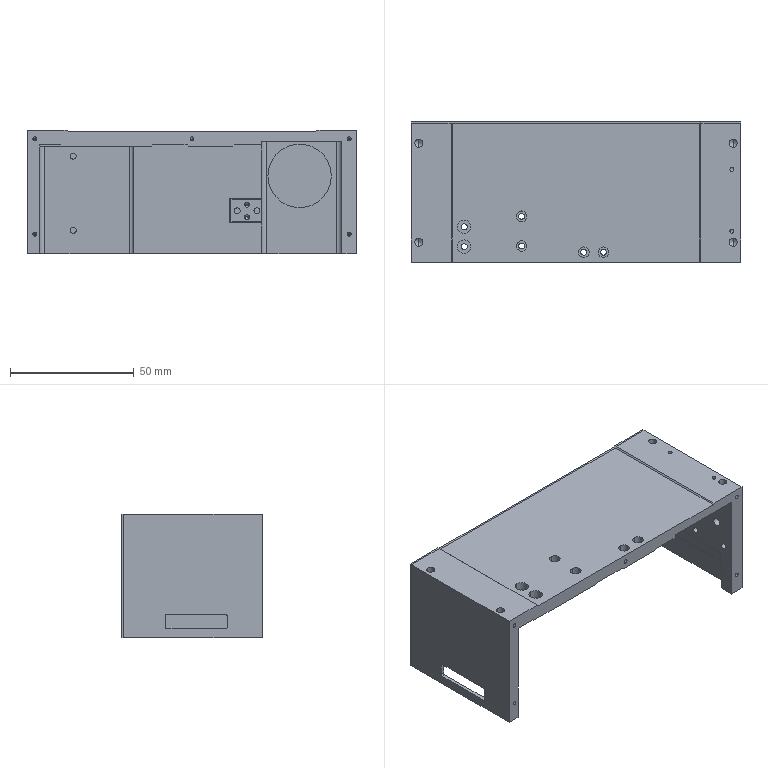NC program | NX | posted with a generic post | part box 133 x 56.74 x 50 mm
Lines 6286 to 7308 of 22463:
(CAVITY_MILL_COPY , TOOL : D6)
N12546 T06 M6
N12548 G54
N12550 G17 G0 G90 X58.566 Y-14.571 B0. C0. S9509 M3
N12552 G43 Z30. H6
N12554 Z1.
N12556 G94 G1 Z-0.5 F1000.
N12558 X59.504 Y-15.367
N12560 G3 X60.488 Y-15.546 R1.
N12562 G2 X61.5 Y-15.37 R3. F1500.
N12564 G1 X62.
N12566 Y-13.594
N12568 G3 X61.5 Y-12.728 R1.
N12570 G1 X60.2 Y-11.977
N12572 Z1.
N12574 G0 Z30.
N12576 X58.566 Y-14.571
N12578 Z0.5
N12580 G1 Z-1. F1000.
N12582 X59.504 Y-15.367
N12584 G3 X60.488 Y-15.546 R1.
N12586 G2 X61.5 Y-15.37 R3. F1500.
N12588 G1 X62.
N12590 Y-13.594
N12592 G3 X61.5 Y-12.728 R1.
N12594 G1 X60.2 Y-11.977
N12596 Z0.5
N12598 G0 Z30.
N12600 X58.566 Y-14.571
N12602 Z0.
N12604 G1 Z-1.5 F1000.
N12606 X59.504 Y-15.367
N12608 G3 X60.488 Y-15.546 R1.
N12610 G2 X61.5 Y-15.37 R3. F1500.
N12612 G1 X62.
N12614 Y-13.594
N12616 G3 X61.5 Y-12.728 R1.
N12618 G1 X60.2 Y-11.977
N12620 Z0.
N12622 G0 X58.566 Y-14.571 Z-0.5
N12624 G1 Z-2. F1000.
N12626 X59.504 Y-15.367
N12628 G3 X60.488 Y-15.546 R1.
N12630 G2 X61.5 Y-15.37 R3. F1500.
N12632 G1 X62.
N12634 Y-13.594
N12636 G3 X61.5 Y-12.728 R1.
N12638 G1 X60.2 Y-11.977
N12640 Z-0.5
N12642 G0 X58.566 Y-14.571 Z-1.
N12644 G1 Z-2.5 F1000.
N12646 X59.504 Y-15.367
N12648 G3 X60.488 Y-15.546 R1.
N12650 G2 X61.5 Y-15.37 R3. F1500.
N12652 G1 X62.
N12654 Y-13.594
N12656 G3 X61.5 Y-12.728 R1.
N12658 G1 X60.2 Y-11.977
N12660 Z-1.
N12662 G0 X58.566 Y-14.571 Z-1.5
N12664 G1 Z-3. F1000.
N12666 X59.504 Y-15.367
N12668 G3 X60.488 Y-15.546 R1.
N12670 G2 X61.5 Y-15.37 R3. F1500.
N12672 G1 X62.
N12674 Y-13.594
N12676 G3 X61.5 Y-12.728 R1.
N12678 G1 X60.2 Y-11.977
N12680 Z-1.5
N12682 G0 X58.566 Y-14.571 Z-2.
N12684 G1 Z-3.5 F1000.
N12686 X59.504 Y-15.367
N12688 G3 X60.488 Y-15.546 R1.
N12690 G2 X61.5 Y-15.37 R3. F1500.
N12692 G1 X62.
N12694 Y-13.594
N12696 G3 X61.5 Y-12.728 R1.
N12698 G1 X60.2 Y-11.977
N12700 Z-2.
N12702 G0 X58.566 Y-14.571 Z-2.5
N12704 G1 Z-4. F1000.
N12706 X59.504 Y-15.367
N12708 G3 X60.488 Y-15.546 R1.
N12710 G2 X61.5 Y-15.37 R3. F1500.
N12712 G1 X62.
N12714 Y-13.594
N12716 G3 X61.5 Y-12.728 R1.
N12718 G1 X60.2 Y-11.977
N12720 Z-2.5
N12722 G0 X58.566 Y-14.571 Z-3.
N12724 G1 Z-4.5 F1000.
N12726 X59.504 Y-15.367
N12728 G3 X60.488 Y-15.546 R1.
N12730 G2 X61.5 Y-15.37 R3. F1500.
N12732 G1 X62.
N12734 Y-13.594
N12736 G3 X61.5 Y-12.728 R1.
N12738 G1 X60.2 Y-11.977
N12740 Z-3.
N12742 G0 X58.566 Y-14.571 Z-3.5
N12744 G1 Z-5. F1000.
N12746 X59.504 Y-15.367
N12748 G3 X60.488 Y-15.546 R1.
N12750 G2 X61.5 Y-15.37 R3. F1500.
N12752 G1 X62.
N12754 Y-13.594
N12756 G3 X61.5 Y-12.728 R1.
N12758 G1 X60.2 Y-11.977
N12760 Z-3.5
N12762 G0 X58.566 Y-14.571 Z-4.
N12764 G1 Z-5.5 F1000.
N12766 X59.504 Y-15.367
N12768 G3 X60.488 Y-15.546 R1.
N12770 G2 X61.5 Y-15.37 R3. F1500.
N12772 G1 X62.
N12774 Y-13.594
N12776 G3 X61.5 Y-12.728 R1.
N12778 G1 X60.2 Y-11.977
N12780 Z-4.
N12782 G0 X58.566 Y-14.571 Z-4.5
N12784 G1 Z-6. F1000.
N12786 X59.504 Y-15.367
N12788 G3 X60.488 Y-15.546 R1.
N12790 G2 X61.5 Y-15.37 R3. F1500.
N12792 G1 X62.
N12794 Y-13.594
N12796 G3 X61.5 Y-12.728 R1.
N12798 G1 X60.2 Y-11.977
N12800 Z-4.5
N12802 G0 X58.566 Y-14.571 Z-5.
N12804 G1 Z-6.5 F1000.
N12806 X59.504 Y-15.367
N12808 G3 X60.488 Y-15.546 R1.
N12810 G2 X61.5 Y-15.37 R3. F1500.
N12812 G1 X62.
N12814 Y-13.594
N12816 G3 X61.5 Y-12.728 R1.
N12818 G1 X60.2 Y-11.977
N12820 Z-5.
N12822 G0 X58.566 Y-14.571 Z-5.5
N12824 G1 Z-7. F1000.
N12826 X59.504 Y-15.367
N12828 G3 X60.488 Y-15.546 R1.
N12830 G2 X61.5 Y-15.37 R3. F1500.
N12832 G1 X62.
N12834 Y-13.594
N12836 G3 X61.5 Y-12.728 R1.
N12838 G1 X60.2 Y-11.977
N12840 Z-5.5
N12842 G0 X58.566 Y-14.571 Z-6.
N12844 G1 Z-7.5 F1000.
N12846 X59.504 Y-15.367
N12848 G3 X60.488 Y-15.546 R1.
N12850 G2 X61.5 Y-15.37 R3. F1500.
N12852 G1 X62.
N12854 Y-13.594
N12856 G3 X61.5 Y-12.728 R1.
N12858 G1 X60.2 Y-11.977
N12860 Z-6.
N12862 G0 X58.566 Y-14.571 Z-6.5
N12864 G1 Z-8. F1000.
N12866 X59.504 Y-15.367
N12868 G3 X60.488 Y-15.546 R1.
N12870 G2 X61.5 Y-15.37 R3. F1500.
N12872 G1 X62.
N12874 Y-13.594
N12876 G3 X61.5 Y-12.728 R1.
N12878 G1 X60.2 Y-11.977
N12880 Z-6.5
N12882 G0 X58.566 Y-14.571 Z-7.
N12884 G1 Z-8.5 F1000.
N12886 X59.504 Y-15.367
N12888 G3 X60.488 Y-15.546 R1.
N12890 G2 X61.5 Y-15.37 R3. F1500.
N12892 G1 X62.
N12894 Y-13.594
N12896 G3 X61.5 Y-12.728 R1.
N12898 G1 X60.2 Y-11.977
N12900 Z-7.
N12902 G0 X58.566 Y-14.571 Z-7.5
N12904 G1 Z-9. F1000.
N12906 X59.504 Y-15.367
N12908 G3 X60.488 Y-15.546 R1.
N12910 G2 X61.5 Y-15.37 R3. F1500.
N12912 G1 X62.
N12914 Y-13.594
N12916 G3 X61.5 Y-12.728 R1.
N12918 G1 X60.2 Y-11.977
N12920 Z-7.5
N12922 G0 X58.566 Y-14.571 Z-8.
N12924 G1 Z-9.5 F1000.
N12926 X59.504 Y-15.367
N12928 G3 X60.488 Y-15.546 R1.
N12930 G2 X61.5 Y-15.37 R3. F1500.
N12932 G1 X62.
N12934 Y-13.594
N12936 G3 X61.5 Y-12.728 R1.
N12938 G1 X60.2 Y-11.977
N12940 Z-8.
N12942 G0 Z30.
N12944 X57.246 Y-35.594
N12946 Z-42.5
N12948 G1 Z-44. F1000.
N12950 X56.815 Y-30.34
N12952 G2 X57.246 Y-29.438 R1.
N12954 X58.196 Y-29.76 R1.56 F1500.
N12956 G3 X58.5 Y-29.863 R0.5
N12958 G1 Y-0.8
N12960 G3 X58.015 Y-1.18 R0.5
N12962 G2 X55.63 Y-2.101 R1.56
N12964 G3 X55.011 Y-2.15 R0.5
N12966 G2 X55.993 Y-4.37 R3.
N12968 G1 Y-29.863
N12970 G3 X56.297 Y-29.76 R0.5
N12972 G2 X57.246 Y-29.438 R1.56
N12974 X58.112 Y-29.938 R1.
N12976 G1 Z-42.5
N12978 G0 Z30.
N12980 X56.7 Y6.007
N12982 Z-42.5
N12984 G1 Z-44. F1000.
N12986 X58. Y6.758
N12988 G3 X58.5 Y7.624 R1.
N12990 G1 Y9.63 F1500.
N12992 X56.494
N12994 G3 X55.628 Y9.13 R1.
N12996 G1 X54.877 Y7.83
N12998 Z-42.5
N13000 G0 Z30.
N13002 X60.2 Y13.237
N13004 Z1.
N13006 G1 Z-0.5 F1000.
N13008 X61.5 Y13.988
N13010 G3 X62. Y14.854 R1.
N13012 G1 Y16.63 F1500.
N13014 X61.5
N13016 G2 X60.488 Y16.806 R3.
N13018 G3 X59.504 Y16.627 R1.
N13020 G1 X58.566 Y15.831
N13022 Z1.
N13024 G0 Z30.
N13026 X60.2 Y13.237
N13028 Z0.5
N13030 G1 Z-1. F1000.
N13032 X61.5 Y13.988
N13034 G3 X62. Y14.854 R1.
N13036 G1 Y16.63 F1500.
N13038 X61.5
N13040 G2 X60.488 Y16.806 R3.
N13042 G3 X59.504 Y16.627 R1.
N13044 G1 X58.566 Y15.831
N13046 Z0.5
N13048 G0 Z30.
N13050 X60.2 Y13.237
N13052 Z0.
N13054 G1 Z-1.5 F1000.
N13056 X61.5 Y13.988
N13058 G3 X62. Y14.854 R1.
N13060 G1 Y16.63 F1500.
N13062 X61.5
N13064 G2 X60.488 Y16.806 R3.
N13066 G3 X59.504 Y16.627 R1.
N13068 G1 X58.566 Y15.831
N13070 Z0.
N13072 G0 X60.2 Y13.237 Z-0.5
N13074 G1 Z-2. F1000.
N13076 X61.5 Y13.988
N13078 G3 X62. Y14.854 R1.
N13080 G1 Y16.63 F1500.
N13082 X61.5
N13084 G2 X60.488 Y16.806 R3.
N13086 G3 X59.504 Y16.627 R1.
N13088 G1 X58.566 Y15.831
N13090 Z-0.5
N13092 G0 X60.2 Y13.237 Z-1.
N13094 G1 Z-2.5 F1000.
N13096 X61.5 Y13.988
N13098 G3 X62. Y14.854 R1.
N13100 G1 Y16.63 F1500.
N13102 X61.5
N13104 G2 X60.488 Y16.806 R3.
N13106 G3 X59.504 Y16.627 R1.
N13108 G1 X58.566 Y15.831
N13110 Z-1.
N13112 G0 X60.2 Y13.237 Z-1.5
N13114 G1 Z-3. F1000.
N13116 X61.5 Y13.988
N13118 G3 X62. Y14.854 R1.
N13120 G1 Y16.63 F1500.
N13122 X61.5
N13124 G2 X60.488 Y16.806 R3.
N13126 G3 X59.504 Y16.627 R1.
N13128 G1 X58.566 Y15.831
N13130 Z-1.5
N13132 G0 X60.2 Y13.237 Z-2.
N13134 G1 Z-3.5 F1000.
N13136 X61.5 Y13.988
N13138 G3 X62. Y14.854 R1.
N13140 G1 Y16.63 F1500.
N13142 X61.5
N13144 G2 X60.488 Y16.806 R3.
N13146 G3 X59.504 Y16.627 R1.
N13148 G1 X58.566 Y15.831
N13150 Z-2.
N13152 G0 X60.2 Y13.237 Z-2.5
N13154 G1 Z-4. F1000.
N13156 X61.5 Y13.988
N13158 G3 X62. Y14.854 R1.
N13160 G1 Y16.63 F1500.
N13162 X61.5
N13164 G2 X60.488 Y16.806 R3.
N13166 G3 X59.504 Y16.627 R1.
N13168 G1 X58.566 Y15.831
N13170 Z-2.5
N13172 G0 X60.2 Y13.237 Z-3.
N13174 G1 Z-4.5 F1000.
N13176 X61.5 Y13.988
N13178 G3 X62. Y14.854 R1.
N13180 G1 Y16.63 F1500.
N13182 X61.5
N13184 G2 X60.488 Y16.806 R3.
N13186 G3 X59.504 Y16.627 R1.
N13188 G1 X58.566 Y15.831
N13190 Z-3.
N13192 G0 X60.2 Y13.237 Z-3.5
N13194 G1 Z-5. F1000.
N13196 X61.5 Y13.988
N13198 G3 X62. Y14.854 R1.
N13200 G1 Y16.63 F1500.
N13202 X61.5
N13204 G2 X60.488 Y16.806 R3.
N13206 G3 X59.504 Y16.627 R1.
N13208 G1 X58.566 Y15.831
N13210 Z-3.5
N13212 G0 X60.2 Y13.237 Z-4.
N13214 G1 Z-5.5 F1000.
N13216 X61.5 Y13.988
N13218 G3 X62. Y14.854 R1.
N13220 G1 Y16.63 F1500.
N13222 X61.5
N13224 G2 X60.488 Y16.806 R3.
N13226 G3 X59.504 Y16.627 R1.
N13228 G1 X58.566 Y15.831
N13230 Z-4.
N13232 G0 X60.2 Y13.237 Z-4.5
N13234 G1 Z-6. F1000.
N13236 X61.5 Y13.988
N13238 G3 X62. Y14.854 R1.
N13240 G1 Y16.63 F1500.
N13242 X61.5
N13244 G2 X60.488 Y16.806 R3.
N13246 G3 X59.504 Y16.627 R1.
N13248 G1 X58.566 Y15.831
N13250 Z-4.5
N13252 G0 X60.2 Y13.237 Z-5.
N13254 G1 Z-6.5 F1000.
N13256 X61.5 Y13.988
N13258 G3 X62. Y14.854 R1.
N13260 G1 Y16.63 F1500.
N13262 X61.5
N13264 G2 X60.488 Y16.806 R3.
N13266 G3 X59.504 Y16.627 R1.
N13268 G1 X58.566 Y15.831
N13270 Z-5.
N13272 G0 X60.2 Y13.237 Z-5.5
N13274 G1 Z-7. F1000.
N13276 X61.5 Y13.988
N13278 G3 X62. Y14.854 R1.
N13280 G1 Y16.63 F1500.
N13282 X61.5
N13284 G2 X60.488 Y16.806 R3.
N13286 G3 X59.504 Y16.627 R1.
N13288 G1 X58.566 Y15.831
N13290 Z-5.5
N13292 G0 X60.2 Y13.237 Z-6.
N13294 G1 Z-7.5 F1000.
N13296 X61.5 Y13.988
N13298 G3 X62. Y14.854 R1.
N13300 G1 Y16.63 F1500.
N13302 X61.5
N13304 G2 X60.488 Y16.806 R3.
N13306 G3 X59.504 Y16.627 R1.
N13308 G1 X58.566 Y15.831
N13310 Z-6.
N13312 G0 X60.2 Y13.237 Z-6.5
N13314 G1 Z-8. F1000.
N13316 X61.5 Y13.988
N13318 G3 X62. Y14.854 R1.
N13320 G1 Y16.63 F1500.
N13322 X61.5
N13324 G2 X60.488 Y16.806 R3.
N13326 G3 X59.504 Y16.627 R1.
N13328 G1 X58.566 Y15.831
N13330 Z-6.5
N13332 G0 X60.2 Y13.237 Z-7.
N13334 G1 Z-8.5 F1000.
N13336 X61.5 Y13.988
N13338 G3 X62. Y14.854 R1.
N13340 G1 Y16.63 F1500.
N13342 X61.5
N13344 G2 X60.488 Y16.806 R3.
N13346 G3 X59.504 Y16.627 R1.
N13348 G1 X58.566 Y15.831
N13350 Z-7.
N13352 G0 X60.2 Y13.237 Z-7.5
N13354 G1 Z-9. F1000.
N13356 X61.5 Y13.988
N13358 G3 X62. Y14.854 R1.
N13360 G1 Y16.63 F1500.
N13362 X61.5
N13364 G2 X60.488 Y16.806 R3.
N13366 G3 X59.504 Y16.627 R1.
N13368 G1 X58.566 Y15.831
N13370 Z-7.5
N13372 G0 X60.2 Y13.237 Z-8.
N13374 G1 Z-9.5 F1000.
N13376 X61.5 Y13.988
N13378 G3 X62. Y14.854 R1.
N13380 G1 Y16.63 F1500.
N13382 X61.5
N13384 G2 X60.488 Y16.806 R3.
N13386 G3 X59.504 Y16.627 R1.
N13388 G1 X58.566 Y15.831
N13390 Z-8.
N13392 G0 Z30.
N13394 X58.036 Y16.307
N13396 Z1.
N13398 G1 Z-0.5 F1000.
N13400 X58.727 Y17.325
N13402 G3 X58.8 Y18.323 R1.
N13404 G2 X58.5 Y19.63 R3. F1500.
N13406 G1 X56.911
N13408 G3 X56.045 Y19.13 R1.
N13410 G1 X55.294 Y17.83
N13412 Z1.
N13414 G0 Z30.
N13416 X58.036 Y16.307
N13418 Z0.5
N13420 G1 Z-1. F1000.
N13422 X58.727 Y17.325
N13424 G3 X58.8 Y18.323 R1.
N13426 G2 X58.5 Y19.63 R3. F1500.
N13428 G1 X56.911
N13430 G3 X56.045 Y19.13 R1.
N13432 G1 X55.294 Y17.83
N13434 Z0.5
N13436 G0 Z30.
N13438 X58.036 Y16.307
N13440 Z0.
N13442 G1 Z-1.5 F1000.
N13444 X58.727 Y17.325
N13446 G3 X58.8 Y18.323 R1.
N13448 G2 X58.5 Y19.63 R3. F1500.
N13450 G1 X56.911
N13452 G3 X56.045 Y19.13 R1.
N13454 G1 X55.294 Y17.83
N13456 Z0.
N13458 G0 X58.036 Y16.307 Z-0.5
N13460 G1 Z-2. F1000.
N13462 X58.727 Y17.325
N13464 G3 X58.8 Y18.323 R1.
N13466 G2 X58.5 Y19.63 R3. F1500.
N13468 G1 X56.911
N13470 G3 X56.045 Y19.13 R1.
N13472 G1 X55.294 Y17.83
N13474 Z-0.5
N13476 G0 X58.036 Y16.307 Z-1.
N13478 G1 Z-2.5 F1000.
N13480 X58.727 Y17.325
N13482 G3 X58.8 Y18.323 R1.
N13484 G2 X58.5 Y19.63 R3. F1500.
N13486 G1 X56.911
N13488 G3 X56.045 Y19.13 R1.
N13490 G1 X55.294 Y17.83
N13492 Z-1.
N13494 G0 X58.036 Y16.307 Z-1.5
N13496 G1 Z-3. F1000.
N13498 X58.727 Y17.325
N13500 G3 X58.8 Y18.323 R1.
N13502 G2 X58.5 Y19.63 R3. F1500.
N13504 G1 X56.911
N13506 G3 X56.045 Y19.13 R1.
N13508 G1 X55.294 Y17.83
N13510 Z-1.5
N13512 G0 X58.036 Y16.307 Z-2.
N13514 G1 Z-3.5 F1000.
N13516 X58.727 Y17.325
N13518 G3 X58.8 Y18.323 R1.
N13520 G2 X58.5 Y19.63 R3. F1500.
N13522 G1 X56.911
N13524 G3 X56.045 Y19.13 R1.
N13526 G1 X55.294 Y17.83
N13528 Z-2.
N13530 G0 X58.036 Y16.307 Z-2.5
N13532 G1 Z-4. F1000.
N13534 X58.727 Y17.325
N13536 G3 X58.8 Y18.323 R1.
N13538 G2 X58.5 Y19.63 R3. F1500.
N13540 G1 X56.911
N13542 G3 X56.045 Y19.13 R1.
N13544 G1 X55.294 Y17.83
N13546 Z-2.5
N13548 G0 X58.036 Y16.307 Z-3.
N13550 G1 Z-4.5 F1000.
N13552 X58.727 Y17.325
N13554 G3 X58.8 Y18.323 R1.
N13556 G2 X58.5 Y19.63 R3. F1500.
N13558 G1 X56.911
N13560 G3 X56.045 Y19.13 R1.
N13562 G1 X55.294 Y17.83
N13564 Z-3.
N13566 G0 X58.036 Y16.307 Z-3.5
N13568 G1 Z-5. F1000.
N13570 X58.727 Y17.325
N13572 G3 X58.8 Y18.323 R1.
N13574 G2 X58.5 Y19.63 R3. F1500.
N13576 G1 X56.911
N13578 G3 X56.045 Y19.13 R1.
N13580 G1 X55.294 Y17.83
N13582 Z-3.5
N13584 G0 X58.036 Y16.307 Z-4.
N13586 G1 Z-5.5 F1000.
N13588 X58.727 Y17.325
N13590 G3 X58.8 Y18.323 R1.
N13592 G2 X58.5 Y19.63 R3. F1500.
N13594 G1 X56.911
N13596 G3 X56.045 Y19.13 R1.
N13598 G1 X55.294 Y17.83
N13600 Z-4.
N13602 G0 X58.036 Y16.307 Z-4.5
N13604 G1 Z-6. F1000.
N13606 X58.727 Y17.325
N13608 G3 X58.8 Y18.323 R1.
N13610 G2 X58.5 Y19.63 R3. F1500.
N13612 G1 X56.911
N13614 G3 X56.045 Y19.13 R1.
N13616 G1 X55.294 Y17.83
N13618 Z-4.5
N13620 G0 X58.036 Y16.307 Z-5.
N13622 G1 Z-6.5 F1000.
N13624 X58.727 Y17.325
N13626 G3 X58.8 Y18.323 R1.
N13628 G2 X58.5 Y19.63 R3. F1500.
N13630 G1 X56.911
N13632 G3 X56.045 Y19.13 R1.
N13634 G1 X55.294 Y17.83
N13636 Z-5.
N13638 G0 X58.036 Y16.307 Z-5.5
N13640 G1 Z-7. F1000.
N13642 X58.727 Y17.325
N13644 G3 X58.8 Y18.323 R1.
N13646 G2 X58.5 Y19.63 R3. F1500.
N13648 G1 X56.911
N13650 G3 X56.045 Y19.13 R1.
N13652 G1 X55.294 Y17.83
N13654 Z-5.5
N13656 G0 X58.036 Y16.307 Z-6.
N13658 G1 Z-7.5 F1000.
N13660 X58.727 Y17.325
N13662 G3 X58.8 Y18.323 R1.
N13664 G2 X58.5 Y19.63 R3. F1500.
N13666 G1 X56.911
N13668 G3 X56.045 Y19.13 R1.
N13670 G1 X55.294 Y17.83
N13672 Z-6.
N13674 G0 X58.036 Y16.307 Z-6.5
N13676 G1 Z-8. F1000.
N13678 X58.727 Y17.325
N13680 G3 X58.8 Y18.323 R1.
N13682 G2 X58.5 Y19.63 R3. F1500.
N13684 G1 X56.911
N13686 G3 X56.045 Y19.13 R1.
N13688 G1 X55.294 Y17.83
N13690 Z-6.5
N13692 G0 X58.036 Y16.307 Z-7.
N13694 G1 Z-8.5 F1000.
N13696 X58.727 Y17.325
N13698 G3 X58.8 Y18.323 R1.
N13700 G2 X58.5 Y19.63 R3. F1500.
N13702 G1 X56.911
N13704 G3 X56.045 Y19.13 R1.
N13706 G1 X55.294 Y17.83
N13708 Z-7.
N13710 G0 X58.036 Y16.307 Z-7.5
N13712 G1 Z-9. F1000.
N13714 X58.727 Y17.325
N13716 G3 X58.8 Y18.323 R1.
N13718 G2 X58.5 Y19.63 R3. F1500.
N13720 G1 X56.911
N13722 G3 X56.045 Y19.13 R1.
N13724 G1 X55.294 Y17.83
N13726 Z-7.5
N13728 G0 X58.036 Y16.307 Z-8.
N13730 G1 Z-9.5 F1000.
N13732 X58.727 Y17.325
N13734 G3 X58.8 Y18.323 R1.
N13736 G2 X58.5 Y19.63 R3. F1500.
N13738 G1 X56.911
N13740 G3 X56.045 Y19.13 R1.
N13742 G1 X55.294 Y17.83
N13744 Z-8.
N13746 G0 X56.7 Y16.007 Z-8.5
N13748 G1 Z-10. F1000.
N13750 X58. Y16.758
N13752 G3 X58.5 Y17.624 R1.
N13754 G1 Y19.63 F1500.
N13756 X56.494
N13758 G3 X55.628 Y19.13 R1.
N13760 G1 X54.877 Y17.83
N13762 Z-8.5
N13764 G0 X56.7 Y16.007 Z-9.
N13766 G1 Z-10.5 F1000.
N13768 X58. Y16.758
N13770 G3 X58.5 Y17.624 R1.
N13772 G1 Y19.63 F1500.
N13774 X56.494
N13776 G3 X55.628 Y19.13 R1.
N13778 G1 X54.877 Y17.83
N13780 Z-9.
N13782 G0 X56.7 Y16.007 Z-9.5
N13784 G1 Z-11. F1000.
N13786 X58. Y16.758
N13788 G3 X58.5 Y17.624 R1.
N13790 G1 Y19.63 F1500.
N13792 X56.494
N13794 G3 X55.628 Y19.13 R1.
N13796 G1 X54.877 Y17.83
N13798 Z-9.5
N13800 G0 X56.7 Y16.007 Z-10.
N13802 G1 Z-11.5 F1000.
N13804 X58. Y16.758
N13806 G3 X58.5 Y17.624 R1.
N13808 G1 Y19.63 F1500.
N13810 X56.494
N13812 G3 X55.628 Y19.13 R1.
N13814 G1 X54.877 Y17.83
N13816 Z-10.
N13818 G0 X56.7 Y16.007 Z-10.5
N13820 G1 Z-12. F1000.
N13822 X58. Y16.758
N13824 G3 X58.5 Y17.624 R1.
N13826 G1 Y19.63 F1500.
N13828 X56.494
N13830 G3 X55.628 Y19.13 R1.
N13832 G1 X54.877 Y17.83
N13834 Z-10.5
N13836 G0 X56.7 Y16.007 Z-11.
N13838 G1 Z-12.5 F1000.
N13840 X58. Y16.758
N13842 G3 X58.5 Y17.624 R1.
N13844 G1 Y19.63 F1500.
N13846 X56.494
N13848 G3 X55.628 Y19.13 R1.
N13850 G1 X54.877 Y17.83
N13852 Z-11.
N13854 G0 X56.7 Y16.007 Z-11.5
N13856 G1 Z-13. F1000.
N13858 X58. Y16.758
N13860 G3 X58.5 Y17.624 R1.
N13862 G1 Y19.63 F1500.
N13864 X56.494
N13866 G3 X55.628 Y19.13 R1.
N13868 G1 X54.877 Y17.83
N13870 Z-11.5
N13872 G0 X56.7 Y16.007 Z-12.
N13874 G1 Z-13.5 F1000.
N13876 X58. Y16.758
N13878 G3 X58.5 Y17.624 R1.
N13880 G1 Y19.63 F1500.
N13882 X56.494
N13884 G3 X55.628 Y19.13 R1.
N13886 G1 X54.877 Y17.83
N13888 Z-12.
N13890 G0 X56.7 Y16.007 Z-12.5
N13892 G1 Z-14. F1000.
N13894 X58. Y16.758
N13896 G3 X58.5 Y17.624 R1.
N13898 G1 Y19.63 F1500.
N13900 X56.494
N13902 G3 X55.628 Y19.13 R1.
N13904 G1 X54.877 Y17.83
N13906 Z-12.5
N13908 G0 X56.7 Y16.007 Z-13.
N13910 G1 Z-14.5 F1000.
N13912 X58. Y16.758
N13914 G3 X58.5 Y17.624 R1.
N13916 G1 Y19.63 F1500.
N13918 X56.494
N13920 G3 X55.628 Y19.13 R1.
N13922 G1 X54.877 Y17.83
N13924 Z-13.
N13926 G0 X56.7 Y16.007 Z-13.5
N13928 G1 Z-15. F1000.
N13930 X58. Y16.758
N13932 G3 X58.5 Y17.624 R1.
N13934 G1 Y19.63 F1500.
N13936 X56.494
N13938 G3 X55.628 Y19.13 R1.
N13940 G1 X54.877 Y17.83
N13942 Z-13.5
N13944 G0 X56.7 Y16.007 Z-14.
N13946 G1 Z-15.5 F1000.
N13948 X58. Y16.758
N13950 G3 X58.5 Y17.624 R1.
N13952 G1 Y19.63 F1500.
N13954 X56.494
N13956 G3 X55.628 Y19.13 R1.
N13958 G1 X54.877 Y17.83
N13960 Z-14.
N13962 G0 X56.7 Y16.007 Z-14.5
N13964 G1 Z-16. F1000.
N13966 X58. Y16.758
N13968 G3 X58.5 Y17.624 R1.
N13970 G1 Y19.63 F1500.
N13972 X56.494
N13974 G3 X55.628 Y19.13 R1.
N13976 G1 X54.877 Y17.83
N13978 Z-14.5
N13980 G0 X56.7 Y16.007 Z-15.
N13982 G1 Z-16.5 F1000.
N13984 X58. Y16.758
N13986 G3 X58.5 Y17.624 R1.
N13988 G1 Y19.63 F1500.
N13990 X56.494
N13992 G3 X55.628 Y19.13 R1.
N13994 G1 X54.877 Y17.83
N13996 Z-15.
N13998 G0 X56.7 Y16.007 Z-15.5
N14000 G1 Z-17. F1000.
N14002 X58. Y16.758
N14004 G3 X58.5 Y17.624 R1.
N14006 G1 Y19.63 F1500.
N14008 X56.494
N14010 G3 X55.628 Y19.13 R1.
N14012 G1 X54.877 Y17.83
N14014 Z-15.5
N14016 G0 X56.7 Y16.007 Z-16.
N14018 G1 Z-17.5 F1000.
N14020 X58. Y16.758
N14022 G3 X58.5 Y17.624 R1.
N14024 G1 Y19.63 F1500.
N14026 X56.494
N14028 G3 X55.628 Y19.13 R1.
N14030 G1 X54.877 Y17.83
N14032 Z-16.
N14034 G0 X56.7 Y16.007 Z-16.5
N14036 G1 Z-18. F1000.
N14038 X58. Y16.758
N14040 G3 X58.5 Y17.624 R1.
N14042 G1 Y19.63 F1500.
N14044 X56.494
N14046 G3 X55.628 Y19.13 R1.
N14048 G1 X54.877 Y17.83
N14050 Z-16.5
N14052 G0 X56.7 Y16.007 Z-17.
N14054 G1 Z-18.5 F1000.
N14056 X58. Y16.758
N14058 G3 X58.5 Y17.624 R1.
N14060 G1 Y19.63 F1500.
N14062 X56.494
N14064 G3 X55.628 Y19.13 R1.
N14066 G1 X54.877 Y17.83
N14068 Z-17.
N14070 G0 X56.7 Y16.007 Z-17.5
N14072 G1 Z-19. F1000.
N14074 X58. Y16.758
N14076 G3 X58.5 Y17.624 R1.
N14078 G1 Y19.63 F1500.
N14080 X56.494
N14082 G3 X55.628 Y19.13 R1.
N14084 G1 X54.877 Y17.83
N14086 Z-17.5
N14088 G0 X56.7 Y16.007 Z-18.
N14090 G1 Z-19.5 F1000.
N14092 X58. Y16.758
N14094 G3 X58.5 Y17.624 R1.
N14096 G1 Y19.63 F1500.
N14098 X56.494
N14100 G3 X55.628 Y19.13 R1.
N14102 G1 X54.877 Y17.83
N14104 Z-18.
N14106 G0 X56.7 Y16.007 Z-18.5
N14108 G1 Z-20. F1000.
N14110 X58. Y16.758
N14112 G3 X58.5 Y17.624 R1.
N14114 G1 Y19.63 F1500.
N14116 X56.494
N14118 G3 X55.628 Y19.13 R1.
N14120 G1 X54.877 Y17.83
N14122 Z-18.5
N14124 G0 X56.7 Y16.007 Z-19.
N14126 G1 Z-20.5 F1000.
N14128 X58. Y16.758
N14130 G3 X58.5 Y17.624 R1.
N14132 G1 Y19.63 F1500.
N14134 X56.494
N14136 G3 X55.628 Y19.13 R1.
N14138 G1 X54.877 Y17.83
N14140 Z-19.
N14142 G0 X56.7 Y16.007 Z-19.5
N14144 G1 Z-21. F1000.
N14146 X58. Y16.758
N14148 G3 X58.5 Y17.624 R1.
N14150 G1 Y19.63 F1500.
N14152 X56.494
N14154 G3 X55.628 Y19.13 R1.
N14156 G1 X54.877 Y17.83
N14158 Z-19.5
N14160 G0 X56.7 Y16.007 Z-20.
N14162 G1 Z-21.5 F1000.
N14164 X58. Y16.758
N14166 G3 X58.5 Y17.624 R1.
N14168 G1 Y19.63 F1500.
N14170 X56.494
N14172 G3 X55.628 Y19.13 R1.
N14174 G1 X54.877 Y17.83
N14176 Z-20.
N14178 G0 X56.7 Y16.007 Z-20.5
N14180 G1 Z-22. F1000.
N14182 X58. Y16.758
N14184 G3 X58.5 Y17.624 R1.
N14186 G1 Y19.63 F1500.
N14188 X56.494
N14190 G3 X55.628 Y19.13 R1.
N14192 G1 X54.877 Y17.83
N14194 Z-20.5
N14196 G0 X56.7 Y16.007 Z-21.
N14198 G1 Z-22.5 F1000.
N14200 X58. Y16.758
N14202 G3 X58.5 Y17.624 R1.
N14204 G1 Y19.63 F1500.
N14206 X56.494
N14208 G3 X55.628 Y19.13 R1.
N14210 G1 X54.877 Y17.83
N14212 Z-21.
N14214 G0 X56.7 Y16.007 Z-21.5
N14216 G1 Z-23. F1000.
N14218 X58. Y16.758
N14220 G3 X58.5 Y17.624 R1.
N14222 G1 Y19.63 F1500.
N14224 X56.494
N14226 G3 X55.628 Y19.13 R1.
N14228 G1 X54.877 Y17.83
N14230 Z-21.5
N14232 G0 X56.7 Y16.007 Z-22.
N14234 G1 Z-23.5 F1000.
N14236 X58. Y16.758
N14238 G3 X58.5 Y17.624 R1.
N14240 G1 Y19.63 F1500.
N14242 X56.494
N14244 G3 X55.628 Y19.13 R1.
N14246 G1 X54.877 Y17.83
N14248 Z-22.
N14250 G0 X56.7 Y16.007 Z-22.5
N14252 G1 Z-24. F1000.
N14254 X58. Y16.758
N14256 G3 X58.5 Y17.624 R1.
N14258 G1 Y19.63 F1500.
N14260 X56.494
N14262 G3 X55.628 Y19.13 R1.
N14264 G1 X54.877 Y17.83
N14266 Z-22.5
N14268 G0 X56.7 Y16.007 Z-23.
N14270 G1 Z-24.5 F1000.
N14272 X58. Y16.758
N14274 G3 X58.5 Y17.624 R1.
N14276 G1 Y19.63 F1500.
N14278 X56.494
N14280 G3 X55.628 Y19.13 R1.
N14282 G1 X54.877 Y17.83
N14284 Z-23.
N14286 G0 X56.7 Y16.007 Z-23.5
N14288 G1 Z-25. F1000.
N14290 X58. Y16.758
N14292 G3 X58.5 Y17.624 R1.
N14294 G1 Y19.63 F1500.
N14296 X56.494
N14298 G3 X55.628 Y19.13 R1.
N14300 G1 X54.877 Y17.83
N14302 Z-23.5
N14304 G0 X56.7 Y16.007 Z-24.
N14306 G1 Z-25.5 F1000.
N14308 X58. Y16.758
N14310 G3 X58.5 Y17.624 R1.
N14312 G1 Y19.63 F1500.
N14314 X56.494
N14316 G3 X55.628 Y19.13 R1.
N14318 G1 X54.877 Y17.83
N14320 Z-24.
N14322 G0 X56.7 Y16.007 Z-24.5
N14324 G1 Z-26. F1000.
N14326 X58. Y16.758
N14328 G3 X58.5 Y17.624 R1.
N14330 G1 Y19.63 F1500.
N14332 X56.494
N14334 G3 X55.628 Y19.13 R1.
N14336 G1 X54.877 Y17.83
N14338 Z-24.5
N14340 G0 X56.7 Y16.007 Z-25.
N14342 G1 Z-26.5 F1000.
N14344 X58. Y16.758
N14346 G3 X58.5 Y17.624 R1.
N14348 G1 Y19.63 F1500.
N14350 X56.494
N14352 G3 X55.628 Y19.13 R1.
N14354 G1 X54.877 Y17.83
N14356 Z-25.
N14358 G0 X56.7 Y16.007 Z-25.5
N14360 G1 Z-27. F1000.
N14362 X58. Y16.758
N14364 G3 X58.5 Y17.624 R1.
N14366 G1 Y19.63 F1500.
N14368 X56.494
N14370 G3 X55.628 Y19.13 R1.
N14372 G1 X54.877 Y17.83
N14374 Z-25.5
N14376 G0 X56.7 Y16.007 Z-26.
N14378 G1 Z-27.5 F1000.
N14380 X58. Y16.758
N14382 G3 X58.5 Y17.624 R1.
N14384 G1 Y19.63 F1500.
N14386 X56.494
N14388 G3 X55.628 Y19.13 R1.
N14390 G1 X54.877 Y17.83
N14392 Z-26.
N14394 G0 X56.7 Y16.007 Z-26.5
N14396 G1 Z-28. F1000.
N14398 X58. Y16.758
N14400 G3 X58.5 Y17.624 R1.
N14402 G1 Y19.63 F1500.
N14404 X56.494
N14406 G3 X55.628 Y19.13 R1.
N14408 G1 X54.877 Y17.83
N14410 Z-26.5
N14412 G0 X56.7 Y16.007 Z-27.
N14414 G1 Z-28.5 F1000.
N14416 X58. Y16.758
N14418 G3 X58.5 Y17.624 R1.
N14420 G1 Y19.63 F1500.
N14422 X56.494
N14424 G3 X55.628 Y19.13 R1.
N14426 G1 X54.877 Y17.83
N14428 Z-27.
N14430 G0 X56.7 Y16.007 Z-27.5
N14432 G1 Z-29. F1000.
N14434 X58. Y16.758
N14436 G3 X58.5 Y17.624 R1.
N14438 G1 Y19.63 F1500.
N14440 X56.494
N14442 G3 X55.628 Y19.13 R1.
N14444 G1 X54.877 Y17.83
N14446 Z-27.5
N14448 G0 X56.7 Y16.007 Z-28.
N14450 G1 Z-29.5 F1000.
N14452 X58. Y16.758
N14454 G3 X58.5 Y17.624 R1.
N14456 G1 Y19.63 F1500.
N14458 X56.494
N14460 G3 X55.628 Y19.13 R1.
N14462 G1 X54.877 Y17.83
N14464 Z-28.
N14466 G0 X56.7 Y16.007 Z-28.5
N14468 G1 Z-30. F1000.
N14470 X58. Y16.758
N14472 G3 X58.5 Y17.624 R1.
N14474 G1 Y19.63 F1500.
N14476 X56.494
N14478 G3 X55.628 Y19.13 R1.
N14480 G1 X54.877 Y17.83
N14482 Z-28.5
N14484 G0 X56.7 Y16.007 Z-29.
N14486 G1 Z-30.5 F1000.
N14488 X58. Y16.758
N14490 G3 X58.5 Y17.624 R1.
N14492 G1 Y19.63 F1500.
N14494 X56.494
N14496 G3 X55.628 Y19.13 R1.
N14498 G1 X54.877 Y17.83
N14500 Z-29.
N14502 G0 X56.7 Y16.007 Z-29.5
N14504 G1 Z-31. F1000.
N14506 X58. Y16.758
N14508 G3 X58.5 Y17.624 R1.
N14510 G1 Y19.63 F1500.
N14512 X56.494
N14514 G3 X55.628 Y19.13 R1.
N14516 G1 X54.877 Y17.83
N14518 Z-29.5
N14520 G0 X56.7 Y16.007 Z-30.
N14522 G1 Z-31.5 F1000.
N14524 X58. Y16.758
N14526 G3 X58.5 Y17.624 R1.
N14528 G1 Y19.63 F1500.
N14530 X56.494
N14532 G3 X55.628 Y19.13 R1.
N14534 G1 X54.877 Y17.83
N14536 Z-30.
N14538 G0 X56.7 Y16.007 Z-30.5
N14540 G1 Z-32. F1000.
N14542 X58. Y16.758
N14544 G3 X58.5 Y17.624 R1.
N14546 G1 Y19.63 F1500.
N14548 X56.494
N14550 G3 X55.628 Y19.13 R1.
N14552 G1 X54.877 Y17.83
N14554 Z-30.5
N14556 G0 X56.7 Y16.007 Z-31.
N14558 G1 Z-32.5 F1000.
N14560 X58. Y16.758
N14562 G3 X58.5 Y17.624 R1.
N14564 G1 Y19.63 F1500.
N14566 X56.494
N14568 G3 X55.628 Y19.13 R1.
N14570 G1 X54.877 Y17.83
N14572 Z-31.
N14574 G0 X56.7 Y16.007 Z-31.5
N14576 G1 Z-33. F1000.
N14578 X58. Y16.758
N14580 G3 X58.5 Y17.624 R1.
N14582 G1 Y19.63 F1500.
N14584 X56.494